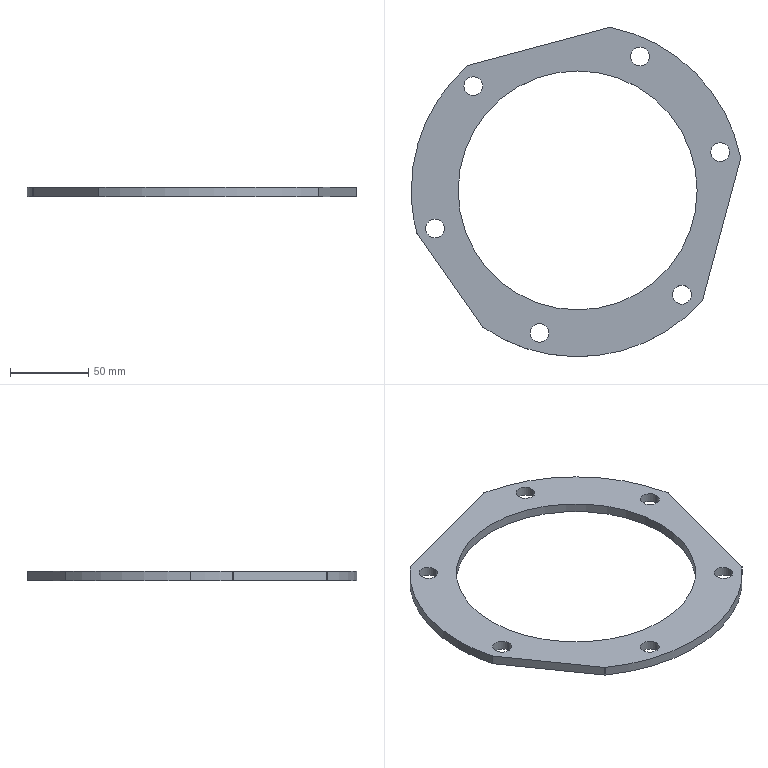Part | SolidWorks | features FlatPattern 1, SMBaseFlange 1, SheetMetal 1 | 1 solid | 29 faces | box 210.92 x 210.92 x 6 mm | volume 89109 mm3 | cylinder 24 | plane 5 | commonest cylinder face diameters 12 x12 2 x6 213 x4 153 x2
STEP:
#1=CARTESIAN_POINT('',(-76.5,0.,6.));
#2=VERTEX_POINT('',#1);
#3=CARTESIAN_POINT('',(76.5,0.,6.));
#4=VERTEX_POINT('',#3);
#5=CARTESIAN_POINT('',(0.,0.,6.));
#6=DIRECTION('',(0.,0.,1.));
#7=DIRECTION('',(1.,0.,0.));
#8=AXIS2_PLACEMENT_3D('',#5,#6,#7);
#9=CIRCLE('',#8,76.5);
#10=EDGE_CURVE('',#2,#4,#9,.T.);
#11=ORIENTED_EDGE('',*,*,#10,.T.);
#12=CARTESIAN_POINT('',(76.5,0.,0.));
#13=VERTEX_POINT('',#12);
#14=CARTESIAN_POINT('',(76.5,0.,6.));
#15=DIRECTION('',(0.,0.,-1.));
#16=VECTOR('',#15,1000.);
#17=LINE('',#14,#16);
#18=EDGE_CURVE('',#4,#13,#17,.T.);
#19=ORIENTED_EDGE('',*,*,#18,.T.);
#20=CARTESIAN_POINT('',(-76.5,0.,0.));
#21=VERTEX_POINT('',#20);
#22=CARTESIAN_POINT('',(0.,0.,0.));
#23=DIRECTION('',(0.,0.,1.));
#24=DIRECTION('',(1.,0.,0.));
#25=AXIS2_PLACEMENT_3D('',#22,#23,#24);
#26=CIRCLE('',#25,76.5);
#27=EDGE_CURVE('',#21,#13,#26,.T.);
#28=ORIENTED_EDGE('',*,*,#27,.F.);
#29=CARTESIAN_POINT('',(-76.5,0.,6.));
#30=DIRECTION('',(0.,0.,-1.));
#31=VECTOR('',#30,1000.);
#32=LINE('',#29,#31);
#33=EDGE_CURVE('',#2,#21,#32,.T.);
#34=ORIENTED_EDGE('',*,*,#33,.F.);
#35=EDGE_LOOP('',(#11,#19,#28,#34));
#36=FACE_OUTER_BOUND('',#35,.T.);
#37=CARTESIAN_POINT('',(0.,0.,6.));
#38=DIRECTION('',(0.,0.,-1.));
#39=DIRECTION('',(-1.,0.,0.));
#40=AXIS2_PLACEMENT_3D('',#37,#38,#39);
#41=CYLINDRICAL_SURFACE('',#40,76.5);
#42=ADVANCED_FACE('',(#36),#41,.F.);
#43=CARTESIAN_POINT('',(-97.28,-24.458,6.));
#44=VERTEX_POINT('',#43);
#45=CARTESIAN_POINT('',(-85.28,-24.458,6.));
#46=VERTEX_POINT('',#45);
#47=CARTESIAN_POINT('',(-91.28,-24.458,6.));
#48=DIRECTION('',(0.,0.,1.));
#49=DIRECTION('',(1.,0.,0.));
#50=AXIS2_PLACEMENT_3D('',#47,#48,#49);
#51=CIRCLE('',#50,6.);
#52=EDGE_CURVE('',#44,#46,#51,.T.);
#53=ORIENTED_EDGE('',*,*,#52,.T.);
#54=CARTESIAN_POINT('',(-85.28,-24.458,0.));
#55=VERTEX_POINT('',#54);
#56=CARTESIAN_POINT('',(-85.28,-24.458,6.));
#57=DIRECTION('',(0.,0.,-1.));
#58=VECTOR('',#57,1000.);
#59=LINE('',#56,#58);
#60=EDGE_CURVE('',#46,#55,#59,.T.);
#61=ORIENTED_EDGE('',*,*,#60,.T.);
#62=CARTESIAN_POINT('',(-97.28,-24.458,0.));
#63=VERTEX_POINT('',#62);
#64=CARTESIAN_POINT('',(-91.28,-24.458,0.));
#65=DIRECTION('',(0.,0.,1.));
#66=DIRECTION('',(1.,0.,0.));
#67=AXIS2_PLACEMENT_3D('',#64,#65,#66);
#68=CIRCLE('',#67,6.);
#69=EDGE_CURVE('',#63,#55,#68,.T.);
#70=ORIENTED_EDGE('',*,*,#69,.F.);
#71=CARTESIAN_POINT('',(-97.28,-24.458,6.));
#72=DIRECTION('',(0.,0.,-1.));
#73=VECTOR('',#72,1000.);
#74=LINE('',#71,#73);
#75=EDGE_CURVE('',#44,#63,#74,.T.);
#76=ORIENTED_EDGE('',*,*,#75,.F.);
#77=EDGE_LOOP('',(#53,#61,#70,#76));
#78=FACE_OUTER_BOUND('',#77,.T.);
#79=CARTESIAN_POINT('',(-91.28,-24.458,6.));
#80=DIRECTION('',(0.,0.,-1.));
#81=DIRECTION('',(-1.,0.,0.));
#82=AXIS2_PLACEMENT_3D('',#79,#80,#81);
#83=CYLINDRICAL_SURFACE('',#82,6.);
#84=ADVANCED_FACE('',(#78),#83,.F.);
#85=CARTESIAN_POINT('',(-30.458,-91.28,6.));
#86=VERTEX_POINT('',#85);
#87=CARTESIAN_POINT('',(-18.458,-91.28,6.));
#88=VERTEX_POINT('',#87);
#89=CARTESIAN_POINT('',(-24.458,-91.28,6.));
#90=DIRECTION('',(0.,0.,1.));
#91=DIRECTION('',(1.,0.,0.));
#92=AXIS2_PLACEMENT_3D('',#89,#90,#91);
#93=CIRCLE('',#92,6.);
#94=EDGE_CURVE('',#86,#88,#93,.T.);
#95=ORIENTED_EDGE('',*,*,#94,.T.);
#96=CARTESIAN_POINT('',(-18.458,-91.28,0.));
#97=VERTEX_POINT('',#96);
#98=CARTESIAN_POINT('',(-18.458,-91.28,6.));
#99=DIRECTION('',(0.,0.,-1.));
#100=VECTOR('',#99,1000.);
#101=LINE('',#98,#100);
#102=EDGE_CURVE('',#88,#97,#101,.T.);
#103=ORIENTED_EDGE('',*,*,#102,.T.);
#104=CARTESIAN_POINT('',(-30.458,-91.28,0.));
#105=VERTEX_POINT('',#104);
#106=CARTESIAN_POINT('',(-24.458,-91.28,0.));
#107=DIRECTION('',(0.,0.,1.));
#108=DIRECTION('',(1.,0.,0.));
#109=AXIS2_PLACEMENT_3D('',#106,#107,#108);
#110=CIRCLE('',#109,6.);
#111=EDGE_CURVE('',#105,#97,#110,.T.);
#112=ORIENTED_EDGE('',*,*,#111,.F.);
#113=CARTESIAN_POINT('',(-30.458,-91.28,6.));
#114=DIRECTION('',(0.,0.,-1.));
#115=VECTOR('',#114,1000.);
#116=LINE('',#113,#115);
#117=EDGE_CURVE('',#86,#105,#116,.T.);
#118=ORIENTED_EDGE('',*,*,#117,.F.);
#119=EDGE_LOOP('',(#95,#103,#112,#118));
#120=FACE_OUTER_BOUND('',#119,.T.);
#121=CARTESIAN_POINT('',(-24.458,-91.28,6.));
#122=DIRECTION('',(0.,0.,-1.));
#123=DIRECTION('',(-1.,0.,0.));
#124=AXIS2_PLACEMENT_3D('',#121,#122,#123);
#125=CYLINDRICAL_SURFACE('',#124,6.);
#126=ADVANCED_FACE('',(#120),#125,.F.);
#127=CARTESIAN_POINT('',(60.822,-66.822,6.));
#128=VERTEX_POINT('',#127);
#129=CARTESIAN_POINT('',(72.822,-66.822,6.));
#130=VERTEX_POINT('',#129);
#131=CARTESIAN_POINT('',(66.822,-66.822,6.));
#132=DIRECTION('',(0.,0.,1.));
#133=DIRECTION('',(1.,0.,0.));
#134=AXIS2_PLACEMENT_3D('',#131,#132,#133);
#135=CIRCLE('',#134,6.);
#136=EDGE_CURVE('',#128,#130,#135,.T.);
#137=ORIENTED_EDGE('',*,*,#136,.T.);
#138=CARTESIAN_POINT('',(72.822,-66.822,0.));
#139=VERTEX_POINT('',#138);
#140=CARTESIAN_POINT('',(72.822,-66.822,6.));
#141=DIRECTION('',(0.,0.,-1.));
#142=VECTOR('',#141,1000.);
#143=LINE('',#140,#142);
#144=EDGE_CURVE('',#130,#139,#143,.T.);
#145=ORIENTED_EDGE('',*,*,#144,.T.);
#146=CARTESIAN_POINT('',(60.822,-66.822,0.));
#147=VERTEX_POINT('',#146);
#148=CARTESIAN_POINT('',(66.822,-66.822,0.));
#149=DIRECTION('',(0.,0.,1.));
#150=DIRECTION('',(1.,0.,0.));
#151=AXIS2_PLACEMENT_3D('',#148,#149,#150);
#152=CIRCLE('',#151,6.);
#153=EDGE_CURVE('',#147,#139,#152,.T.);
#154=ORIENTED_EDGE('',*,*,#153,.F.);
#155=CARTESIAN_POINT('',(60.822,-66.822,6.));
#156=DIRECTION('',(0.,0.,-1.));
#157=VECTOR('',#156,1000.);
#158=LINE('',#155,#157);
#159=EDGE_CURVE('',#128,#147,#158,.T.);
#160=ORIENTED_EDGE('',*,*,#159,.F.);
#161=EDGE_LOOP('',(#137,#145,#154,#160));
#162=FACE_OUTER_BOUND('',#161,.T.);
#163=CARTESIAN_POINT('',(66.822,-66.822,6.));
#164=DIRECTION('',(0.,0.,-1.));
#165=DIRECTION('',(-1.,0.,0.));
#166=AXIS2_PLACEMENT_3D('',#163,#164,#165);
#167=CYLINDRICAL_SURFACE('',#166,6.);
#168=ADVANCED_FACE('',(#162),#167,.F.);
#169=CARTESIAN_POINT('',(85.28,24.458,6.));
#170=VERTEX_POINT('',#169);
#171=CARTESIAN_POINT('',(97.28,24.458,6.));
#172=VERTEX_POINT('',#171);
#173=CARTESIAN_POINT('',(91.28,24.458,6.));
#174=DIRECTION('',(0.,0.,1.));
#175=DIRECTION('',(1.,0.,0.));
#176=AXIS2_PLACEMENT_3D('',#173,#174,#175);
#177=CIRCLE('',#176,6.);
#178=EDGE_CURVE('',#170,#172,#177,.T.);
#179=ORIENTED_EDGE('',*,*,#178,.T.);
#180=CARTESIAN_POINT('',(97.28,24.458,0.));
#181=VERTEX_POINT('',#180);
#182=CARTESIAN_POINT('',(97.28,24.458,6.));
#183=DIRECTION('',(0.,0.,-1.));
#184=VECTOR('',#183,1000.);
#185=LINE('',#182,#184);
#186=EDGE_CURVE('',#172,#181,#185,.T.);
#187=ORIENTED_EDGE('',*,*,#186,.T.);
#188=CARTESIAN_POINT('',(85.28,24.458,0.));
#189=VERTEX_POINT('',#188);
#190=CARTESIAN_POINT('',(91.28,24.458,0.));
#191=DIRECTION('',(0.,0.,1.));
#192=DIRECTION('',(1.,0.,0.));
#193=AXIS2_PLACEMENT_3D('',#190,#191,#192);
#194=CIRCLE('',#193,6.);
#195=EDGE_CURVE('',#189,#181,#194,.T.);
#196=ORIENTED_EDGE('',*,*,#195,.F.);
#197=CARTESIAN_POINT('',(85.28,24.458,6.));
#198=DIRECTION('',(0.,0.,-1.));
#199=VECTOR('',#198,1000.);
#200=LINE('',#197,#199);
#201=EDGE_CURVE('',#170,#189,#200,.T.);
#202=ORIENTED_EDGE('',*,*,#201,.F.);
#203=EDGE_LOOP('',(#179,#187,#196,#202));
#204=FACE_OUTER_BOUND('',#203,.T.);
#205=CARTESIAN_POINT('',(91.28,24.458,6.));
#206=DIRECTION('',(0.,0.,-1.));
#207=DIRECTION('',(-1.,0.,0.));
#208=AXIS2_PLACEMENT_3D('',#205,#206,#207);
#209=CYLINDRICAL_SURFACE('',#208,6.);
#210=ADVANCED_FACE('',(#204),#209,.F.);
#211=CARTESIAN_POINT('',(33.937,85.646,6.));
#212=VERTEX_POINT('',#211);
#213=CARTESIAN_POINT('',(45.937,85.646,6.));
#214=VERTEX_POINT('',#213);
#215=CARTESIAN_POINT('',(39.937,85.646,6.));
#216=DIRECTION('',(0.,0.,1.));
#217=DIRECTION('',(1.,0.,0.));
#218=AXIS2_PLACEMENT_3D('',#215,#216,#217);
#219=CIRCLE('',#218,6.);
#220=EDGE_CURVE('',#212,#214,#219,.T.);
#221=ORIENTED_EDGE('',*,*,#220,.T.);
#222=CARTESIAN_POINT('',(45.937,85.646,0.));
#223=VERTEX_POINT('',#222);
#224=CARTESIAN_POINT('',(45.937,85.646,6.));
#225=DIRECTION('',(0.,0.,-1.));
#226=VECTOR('',#225,1000.);
#227=LINE('',#224,#226);
#228=EDGE_CURVE('',#214,#223,#227,.T.);
#229=ORIENTED_EDGE('',*,*,#228,.T.);
#230=CARTESIAN_POINT('',(33.937,85.646,0.));
#231=VERTEX_POINT('',#230);
#232=CARTESIAN_POINT('',(39.937,85.646,0.));
#233=DIRECTION('',(0.,0.,1.));
#234=DIRECTION('',(1.,0.,0.));
#235=AXIS2_PLACEMENT_3D('',#232,#233,#234);
#236=CIRCLE('',#235,6.);
#237=EDGE_CURVE('',#231,#223,#236,.T.);
#238=ORIENTED_EDGE('',*,*,#237,.F.);
#239=CARTESIAN_POINT('',(33.937,85.646,6.));
#240=DIRECTION('',(0.,0.,-1.));
#241=VECTOR('',#240,1000.);
#242=LINE('',#239,#241);
#243=EDGE_CURVE('',#212,#231,#242,.T.);
#244=ORIENTED_EDGE('',*,*,#243,.F.);
#245=EDGE_LOOP('',(#221,#229,#238,#244));
#246=FACE_OUTER_BOUND('',#245,.T.);
#247=CARTESIAN_POINT('',(39.937,85.646,6.));
#248=DIRECTION('',(0.,0.,-1.));
#249=DIRECTION('',(-1.,0.,0.));
#250=AXIS2_PLACEMENT_3D('',#247,#248,#249);
#251=CYLINDRICAL_SURFACE('',#250,6.);
#252=ADVANCED_FACE('',(#246),#251,.F.);
#253=CARTESIAN_POINT('',(-72.822,66.822,6.));
#254=VERTEX_POINT('',#253);
#255=CARTESIAN_POINT('',(-60.822,66.822,6.));
#256=VERTEX_POINT('',#255);
#257=CARTESIAN_POINT('',(-66.822,66.822,6.));
#258=DIRECTION('',(0.,0.,1.));
#259=DIRECTION('',(1.,0.,0.));
#260=AXIS2_PLACEMENT_3D('',#257,#258,#259);
#261=CIRCLE('',#260,6.);
#262=EDGE_CURVE('',#254,#256,#261,.T.);
#263=ORIENTED_EDGE('',*,*,#262,.T.);
#264=CARTESIAN_POINT('',(-60.822,66.822,0.));
#265=VERTEX_POINT('',#264);
#266=CARTESIAN_POINT('',(-60.822,66.822,6.));
#267=DIRECTION('',(0.,0.,-1.));
#268=VECTOR('',#267,1000.);
#269=LINE('',#266,#268);
#270=EDGE_CURVE('',#256,#265,#269,.T.);
#271=ORIENTED_EDGE('',*,*,#270,.T.);
#272=CARTESIAN_POINT('',(-72.822,66.822,0.));
#273=VERTEX_POINT('',#272);
#274=CARTESIAN_POINT('',(-66.822,66.822,0.));
#275=DIRECTION('',(0.,0.,1.));
#276=DIRECTION('',(1.,0.,0.));
#277=AXIS2_PLACEMENT_3D('',#274,#275,#276);
#278=CIRCLE('',#277,6.);
#279=EDGE_CURVE('',#273,#265,#278,.T.);
#280=ORIENTED_EDGE('',*,*,#279,.F.);
#281=CARTESIAN_POINT('',(-72.822,66.822,6.));
#282=DIRECTION('',(0.,0.,-1.));
#283=VECTOR('',#282,1000.);
#284=LINE('',#281,#283);
#285=EDGE_CURVE('',#254,#273,#284,.T.);
#286=ORIENTED_EDGE('',*,*,#285,.F.);
#287=EDGE_LOOP('',(#263,#271,#280,#286));
#288=FACE_OUTER_BOUND('',#287,.T.);
#289=CARTESIAN_POINT('',(-66.822,66.822,6.));
#290=DIRECTION('',(0.,0.,-1.));
#291=DIRECTION('',(-1.,0.,0.));
#292=AXIS2_PLACEMENT_3D('',#289,#290,#291);
#293=CYLINDRICAL_SURFACE('',#292,6.);
#294=ADVANCED_FACE('',(#288),#293,.F.);
#295=CARTESIAN_POINT('',(-106.5,0.,6.));
#296=VERTEX_POINT('',#295);
#297=CARTESIAN_POINT('',(-102.975,-27.174,6.));
#298=VERTEX_POINT('',#297);
#299=CARTESIAN_POINT('',(0.,0.,6.));
#300=DIRECTION('',(0.,0.,1.));
#301=DIRECTION('',(1.,0.,0.));
#302=AXIS2_PLACEMENT_3D('',#299,#300,#301);
#303=CIRCLE('',#302,106.5);
#304=EDGE_CURVE('',#296,#298,#303,.T.);
#305=ORIENTED_EDGE('',*,*,#304,.F.);
#306=CARTESIAN_POINT('',(-106.5,0.,0.));
#307=VERTEX_POINT('',#306);
#308=CARTESIAN_POINT('',(-106.5,0.,6.));
#309=DIRECTION('',(0.,0.,-1.));
#310=VECTOR('',#309,1000.);
#311=LINE('',#308,#310);
#312=EDGE_CURVE('',#296,#307,#311,.T.);
#313=ORIENTED_EDGE('',*,*,#312,.T.);
#314=CARTESIAN_POINT('',(-102.975,-27.174,0.));
#315=VERTEX_POINT('',#314);
#316=CARTESIAN_POINT('',(0.,0.,0.));
#317=DIRECTION('',(0.,0.,1.));
#318=DIRECTION('',(1.,0.,0.));
#319=AXIS2_PLACEMENT_3D('',#316,#317,#318);
#320=CIRCLE('',#319,106.5);
#321=EDGE_CURVE('',#307,#315,#320,.T.);
#322=ORIENTED_EDGE('',*,*,#321,.T.);
#323=CARTESIAN_POINT('',(-102.975,-27.174,6.));
#324=DIRECTION('',(0.,0.,-1.));
#325=VECTOR('',#324,1000.);
#326=LINE('',#323,#325);
#327=EDGE_CURVE('',#298,#315,#326,.T.);
#328=ORIENTED_EDGE('',*,*,#327,.F.);
#329=EDGE_LOOP('',(#305,#313,#322,#328));
#330=FACE_OUTER_BOUND('',#329,.T.);
#331=CARTESIAN_POINT('',(0.,0.,6.));
#332=DIRECTION('',(0.,0.,-1.));
#333=DIRECTION('',(-1.,0.,0.));
#334=AXIS2_PLACEMENT_3D('',#331,#332,#333);
#335=CYLINDRICAL_SURFACE('',#334,106.5);
#336=ADVANCED_FACE('',(#330),#335,.T.);
#337=ORIENTED_EDGE('',*,*,#52,.F.);
#338=CARTESIAN_POINT('',(-91.28,-24.458,6.));
#339=DIRECTION('',(0.,0.,1.));
#340=DIRECTION('',(1.,0.,0.));
#341=AXIS2_PLACEMENT_3D('',#338,#339,#340);
#342=CIRCLE('',#341,6.);
#343=EDGE_CURVE('',#46,#44,#342,.T.);
#344=ORIENTED_EDGE('',*,*,#343,.F.);
#345=EDGE_LOOP('',(#337,#344));
#346=FACE_BOUND('',#345,.T.);
#347=ORIENTED_EDGE('',*,*,#136,.F.);
#348=CARTESIAN_POINT('',(66.822,-66.822,6.));
#349=DIRECTION('',(0.,0.,1.));
#350=DIRECTION('',(1.,0.,0.));
#351=AXIS2_PLACEMENT_3D('',#348,#349,#350);
#352=CIRCLE('',#351,6.);
#353=EDGE_CURVE('',#130,#128,#352,.T.);
#354=ORIENTED_EDGE('',*,*,#353,.F.);
#355=EDGE_LOOP('',(#347,#354));
#356=FACE_BOUND('',#355,.T.);
#357=ORIENTED_EDGE('',*,*,#220,.F.);
#358=CARTESIAN_POINT('',(39.937,85.646,6.));
#359=DIRECTION('',(0.,0.,1.));
#360=DIRECTION('',(1.,0.,0.));
#361=AXIS2_PLACEMENT_3D('',#358,#359,#360);
#362=CIRCLE('',#361,6.);
#363=EDGE_CURVE('',#214,#212,#362,.T.);
#364=ORIENTED_EDGE('',*,*,#363,.F.);
#365=EDGE_LOOP('',(#357,#364));
#366=FACE_BOUND('',#365,.T.);
#367=CARTESIAN_POINT('',(-70.023,80.106,6.));
#368=VERTEX_POINT('',#367);
#369=CARTESIAN_POINT('',(-70.426,79.89,6.));
#370=VERTEX_POINT('',#369);
#371=CARTESIAN_POINT('',(-69.764,79.14,6.));
#372=DIRECTION('',(0.,0.,1.));
#373=DIRECTION('',(1.,0.,0.));
#374=AXIS2_PLACEMENT_3D('',#371,#372,#373);
#375=CIRCLE('',#374,1.);
#376=EDGE_CURVE('',#368,#370,#375,.T.);
#377=ORIENTED_EDGE('',*,*,#376,.T.);
#378=CARTESIAN_POINT('',(0.,0.,6.));
#379=DIRECTION('',(0.,0.,1.));
#380=DIRECTION('',(1.,0.,0.));
#381=AXIS2_PLACEMENT_3D('',#378,#379,#380);
#382=CIRCLE('',#381,106.5);
#383=EDGE_CURVE('',#370,#296,#382,.T.);
#384=ORIENTED_EDGE('',*,*,#383,.T.);
#385=ORIENTED_EDGE('',*,*,#304,.T.);
#386=CARTESIAN_POINT('',(-102.827,-27.492,6.));
#387=VERTEX_POINT('',#386);
#388=CARTESIAN_POINT('',(-102.008,-26.919,6.));
#389=DIRECTION('',(0.,0.,1.));
#390=DIRECTION('',(1.,0.,0.));
#391=AXIS2_PLACEMENT_3D('',#388,#389,#390);
#392=CIRCLE('',#391,1.);
#393=EDGE_CURVE('',#298,#387,#392,.T.);
#394=ORIENTED_EDGE('',*,*,#393,.T.);
#395=CARTESIAN_POINT('',(-61.003,-87.223,6.));
#396=VERTEX_POINT('',#395);
#397=CARTESIAN_POINT('',(-102.827,-27.492,6.));
#398=DIRECTION('',(0.5736,-0.8192,0.));
#399=VECTOR('',#398,1000.);
#400=LINE('',#397,#399);
#401=EDGE_CURVE('',#387,#396,#400,.T.);
#402=ORIENTED_EDGE('',*,*,#401,.T.);
#403=CARTESIAN_POINT('',(-60.755,-87.471,6.));
#404=VERTEX_POINT('',#403);
#405=CARTESIAN_POINT('',(-60.184,-86.649,6.));
#406=DIRECTION('',(0.,0.,1.));
#407=DIRECTION('',(1.,0.,0.));
#408=AXIS2_PLACEMENT_3D('',#405,#406,#407);
#409=CIRCLE('',#408,1.);
#410=EDGE_CURVE('',#396,#404,#409,.T.);
#411=ORIENTED_EDGE('',*,*,#410,.T.);
#412=CARTESIAN_POINT('',(79.89,-70.426,6.));
#413=VERTEX_POINT('',#412);
#414=CARTESIAN_POINT('',(0.,0.,6.));
#415=DIRECTION('',(0.,0.,1.));
#416=DIRECTION('',(1.,0.,0.));
#417=AXIS2_PLACEMENT_3D('',#414,#415,#416);
#418=CIRCLE('',#417,106.5);
#419=EDGE_CURVE('',#404,#413,#418,.T.);
#420=ORIENTED_EDGE('',*,*,#419,.T.);
#421=CARTESIAN_POINT('',(80.106,-70.023,6.));
#422=VERTEX_POINT('',#421);
#423=CARTESIAN_POINT('',(79.14,-69.764,6.));
#424=DIRECTION('',(0.,0.,1.));
#425=DIRECTION('',(1.,0.,0.));
#426=AXIS2_PLACEMENT_3D('',#423,#424,#425);
#427=CIRCLE('',#426,1.);
#428=EDGE_CURVE('',#413,#422,#427,.T.);
#429=ORIENTED_EDGE('',*,*,#428,.T.);
#430=CARTESIAN_POINT('',(104.386,20.589,6.));
#431=VERTEX_POINT('',#430);
#432=CARTESIAN_POINT('',(80.106,-70.023,6.));
#433=DIRECTION('',(0.2588,0.9659,0.));
#434=VECTOR('',#433,1000.);
#435=LINE('',#432,#434);
#436=EDGE_CURVE('',#422,#431,#435,.T.);
#437=ORIENTED_EDGE('',*,*,#436,.T.);
#438=CARTESIAN_POINT('',(104.4,21.045,6.));
#439=VERTEX_POINT('',#438);
#440=CARTESIAN_POINT('',(103.42,20.848,6.));
#441=DIRECTION('',(0.,0.,1.));
#442=DIRECTION('',(1.,0.,0.));
#443=AXIS2_PLACEMENT_3D('',#440,#441,#442);
#444=CIRCLE('',#443,1.);
#445=EDGE_CURVE('',#431,#439,#444,.T.);
#446=ORIENTED_EDGE('',*,*,#445,.T.);
#447=CARTESIAN_POINT('',(21.045,104.4,6.));
#448=VERTEX_POINT('',#447);
#449=CARTESIAN_POINT('',(0.,0.,6.));
#450=DIRECTION('',(0.,0.,1.));
#451=DIRECTION('',(1.,0.,0.));
#452=AXIS2_PLACEMENT_3D('',#449,#450,#451);
#453=CIRCLE('',#452,106.5);
#454=EDGE_CURVE('',#439,#448,#453,.T.);
#455=ORIENTED_EDGE('',*,*,#454,.T.);
#456=CARTESIAN_POINT('',(20.589,104.386,6.));
#457=VERTEX_POINT('',#456);
#458=CARTESIAN_POINT('',(20.848,103.42,6.));
#459=DIRECTION('',(0.,0.,1.));
#460=DIRECTION('',(1.,0.,0.));
#461=AXIS2_PLACEMENT_3D('',#458,#459,#460);
#462=CIRCLE('',#461,1.);
#463=EDGE_CURVE('',#448,#457,#462,.T.);
#464=ORIENTED_EDGE('',*,*,#463,.T.);
#465=CARTESIAN_POINT('',(20.589,104.386,6.));
#466=DIRECTION('',(-0.9659,-0.2588,0.));
#467=VECTOR('',#466,1000.);
#468=LINE('',#465,#467);
#469=EDGE_CURVE('',#457,#368,#468,.T.);
#470=ORIENTED_EDGE('',*,*,#469,.T.);
#471=EDGE_LOOP('',(#377,#384,#385,#394,#402,#411,#420,#429,#437,#446,#455,#464,#470));
#472=FACE_OUTER_BOUND('',#471,.T.);
#473=ORIENTED_EDGE('',*,*,#262,.F.);
#474=CARTESIAN_POINT('',(-66.822,66.822,6.));
#475=DIRECTION('',(0.,0.,1.));
#476=DIRECTION('',(1.,0.,0.));
#477=AXIS2_PLACEMENT_3D('',#474,#475,#476);
#478=CIRCLE('',#477,6.);
#479=EDGE_CURVE('',#256,#254,#478,.T.);
#480=ORIENTED_EDGE('',*,*,#479,.F.);
#481=EDGE_LOOP('',(#473,#480));
#482=FACE_BOUND('',#481,.T.);
#483=ORIENTED_EDGE('',*,*,#178,.F.);
#484=CARTESIAN_POINT('',(91.28,24.458,6.));
#485=DIRECTION('',(0.,0.,1.));
#486=DIRECTION('',(1.,0.,0.));
#487=AXIS2_PLACEMENT_3D('',#484,#485,#486);
#488=CIRCLE('',#487,6.);
#489=EDGE_CURVE('',#172,#170,#488,.T.);
#490=ORIENTED_EDGE('',*,*,#489,.F.);
#491=EDGE_LOOP('',(#483,#490));
#492=FACE_BOUND('',#491,.T.);
#493=ORIENTED_EDGE('',*,*,#94,.F.);
#494=CARTESIAN_POINT('',(-24.458,-91.28,6.));
#495=DIRECTION('',(0.,0.,1.));
#496=DIRECTION('',(1.,0.,0.));
#497=AXIS2_PLACEMENT_3D('',#494,#495,#496);
#498=CIRCLE('',#497,6.);
#499=EDGE_CURVE('',#88,#86,#498,.T.);
#500=ORIENTED_EDGE('',*,*,#499,.F.);
#501=EDGE_LOOP('',(#493,#500));
#502=FACE_BOUND('',#501,.T.);
#503=ORIENTED_EDGE('',*,*,#10,.F.);
#504=CARTESIAN_POINT('',(0.,0.,6.));
#505=DIRECTION('',(0.,0.,1.));
#506=DIRECTION('',(1.,0.,0.));
#507=AXIS2_PLACEMENT_3D('',#504,#505,#506);
#508=CIRCLE('',#507,76.5);
#509=EDGE_CURVE('',#4,#2,#508,.T.);
#510=ORIENTED_EDGE('',*,*,#509,.F.);
#511=EDGE_LOOP('',(#503,#510));
#512=FACE_BOUND('',#511,.T.);
#513=CARTESIAN_POINT('',(-69.764,79.14,6.));
#514=DIRECTION('',(0.,0.,1.));
#515=DIRECTION('',(1.,0.,0.));
#516=AXIS2_PLACEMENT_3D('',#513,#514,#515);
#517=PLANE('',#516);
#518=ADVANCED_FACE('',(#346,#356,#366,#472,#482,#492,#502,#512),#517,.T.);
#519=CARTESIAN_POINT('',(-70.023,80.106,0.));
#520=VERTEX_POINT('',#519);
#521=CARTESIAN_POINT('',(-70.426,79.89,0.));
#522=VERTEX_POINT('',#521);
#523=CARTESIAN_POINT('',(-69.764,79.14,0.));
#524=DIRECTION('',(0.,0.,1.));
#525=DIRECTION('',(1.,0.,0.));
#526=AXIS2_PLACEMENT_3D('',#523,#524,#525);
#527=CIRCLE('',#526,1.);
#528=EDGE_CURVE('',#520,#522,#527,.T.);
#529=ORIENTED_EDGE('',*,*,#528,.F.);
#530=CARTESIAN_POINT('',(20.589,104.386,0.));
#531=VERTEX_POINT('',#530);
#532=CARTESIAN_POINT('',(20.589,104.386,0.));
#533=DIRECTION('',(-0.9659,-0.2588,0.));
#534=VECTOR('',#533,1000.);
#535=LINE('',#532,#534);
#536=EDGE_CURVE('',#531,#520,#535,.T.);
#537=ORIENTED_EDGE('',*,*,#536,.F.);
#538=CARTESIAN_POINT('',(21.045,104.4,0.));
#539=VERTEX_POINT('',#538);
#540=CARTESIAN_POINT('',(20.848,103.42,0.));
#541=DIRECTION('',(0.,0.,1.));
#542=DIRECTION('',(1.,0.,0.));
#543=AXIS2_PLACEMENT_3D('',#540,#541,#542);
#544=CIRCLE('',#543,1.);
#545=EDGE_CURVE('',#539,#531,#544,.T.);
#546=ORIENTED_EDGE('',*,*,#545,.F.);
#547=CARTESIAN_POINT('',(104.4,21.045,0.));
#548=VERTEX_POINT('',#547);
#549=CARTESIAN_POINT('',(0.,0.,0.));
#550=DIRECTION('',(0.,0.,1.));
#551=DIRECTION('',(1.,0.,0.));
#552=AXIS2_PLACEMENT_3D('',#549,#550,#551);
#553=CIRCLE('',#552,106.5);
#554=EDGE_CURVE('',#548,#539,#553,.T.);
#555=ORIENTED_EDGE('',*,*,#554,.F.);
#556=CARTESIAN_POINT('',(104.386,20.589,0.));
#557=VERTEX_POINT('',#556);
#558=CARTESIAN_POINT('',(103.42,20.848,0.));
#559=DIRECTION('',(0.,0.,1.));
#560=DIRECTION('',(1.,0.,0.));
#561=AXIS2_PLACEMENT_3D('',#558,#559,#560);
#562=CIRCLE('',#561,1.);
#563=EDGE_CURVE('',#557,#548,#562,.T.);
#564=ORIENTED_EDGE('',*,*,#563,.F.);
#565=CARTESIAN_POINT('',(80.106,-70.023,0.));
#566=VERTEX_POINT('',#565);
#567=CARTESIAN_POINT('',(80.106,-70.023,0.));
#568=DIRECTION('',(0.2588,0.9659,0.));
#569=VECTOR('',#568,1000.);
#570=LINE('',#567,#569);
#571=EDGE_CURVE('',#566,#557,#570,.T.);
#572=ORIENTED_EDGE('',*,*,#571,.F.);
#573=CARTESIAN_POINT('',(79.89,-70.426,0.));
#574=VERTEX_POINT('',#573);
#575=CARTESIAN_POINT('',(79.14,-69.764,0.));
#576=DIRECTION('',(0.,0.,1.));
#577=DIRECTION('',(1.,0.,0.));
#578=AXIS2_PLACEMENT_3D('',#575,#576,#577);
#579=CIRCLE('',#578,1.);
#580=EDGE_CURVE('',#574,#566,#579,.T.);
#581=ORIENTED_EDGE('',*,*,#580,.F.);
#582=CARTESIAN_POINT('',(-60.755,-87.471,0.));
#583=VERTEX_POINT('',#582);
#584=CARTESIAN_POINT('',(0.,0.,0.));
#585=DIRECTION('',(0.,0.,1.));
#586=DIRECTION('',(1.,0.,0.));
#587=AXIS2_PLACEMENT_3D('',#584,#585,#586);
#588=CIRCLE('',#587,106.5);
#589=EDGE_CURVE('',#583,#574,#588,.T.);
#590=ORIENTED_EDGE('',*,*,#589,.F.);
#591=CARTESIAN_POINT('',(-61.003,-87.223,0.));
#592=VERTEX_POINT('',#591);
#593=CARTESIAN_POINT('',(-60.184,-86.649,0.));
#594=DIRECTION('',(0.,0.,1.));
#595=DIRECTION('',(1.,0.,0.));
#596=AXIS2_PLACEMENT_3D('',#593,#594,#595);
#597=CIRCLE('',#596,1.);
#598=EDGE_CURVE('',#592,#583,#597,.T.);
#599=ORIENTED_EDGE('',*,*,#598,.F.);
#600=CARTESIAN_POINT('',(-102.827,-27.492,0.));
#601=VERTEX_POINT('',#600);
#602=CARTESIAN_POINT('',(-102.827,-27.492,0.));
#603=DIRECTION('',(0.5736,-0.8192,0.));
#604=VECTOR('',#603,1000.);
#605=LINE('',#602,#604);
#606=EDGE_CURVE('',#601,#592,#605,.T.);
#607=ORIENTED_EDGE('',*,*,#606,.F.);
#608=CARTESIAN_POINT('',(-102.008,-26.919,0.));
#609=DIRECTION('',(0.,0.,1.));
#610=DIRECTION('',(1.,0.,0.));
#611=AXIS2_PLACEMENT_3D('',#608,#609,#610);
#612=CIRCLE('',#611,1.);
#613=EDGE_CURVE('',#315,#601,#612,.T.);
#614=ORIENTED_EDGE('',*,*,#613,.F.);
#615=ORIENTED_EDGE('',*,*,#321,.F.);
#616=CARTESIAN_POINT('',(0.,0.,0.));
#617=DIRECTION('',(0.,0.,1.));
#618=DIRECTION('',(1.,0.,0.));
#619=AXIS2_PLACEMENT_3D('',#616,#617,#618);
#620=CIRCLE('',#619,106.5);
#621=EDGE_CURVE('',#522,#307,#620,.T.);
#622=ORIENTED_EDGE('',*,*,#621,.F.);
#623=EDGE_LOOP('',(#529,#537,#546,#555,#564,#572,#581,#590,#599,#607,#614,#615,#622));
#624=FACE_OUTER_BOUND('',#623,.T.);
#625=ORIENTED_EDGE('',*,*,#279,.T.);
#626=CARTESIAN_POINT('',(-66.822,66.822,0.));
#627=DIRECTION('',(0.,0.,1.));
#628=DIRECTION('',(1.,0.,0.));
#629=AXIS2_PLACEMENT_3D('',#626,#627,#628);
#630=CIRCLE('',#629,6.);
#631=EDGE_CURVE('',#265,#273,#630,.T.);
#632=ORIENTED_EDGE('',*,*,#631,.T.);
#633=EDGE_LOOP('',(#625,#632));
#634=FACE_BOUND('',#633,.T.);
#635=ORIENTED_EDGE('',*,*,#237,.T.);
#636=CARTESIAN_POINT('',(39.937,85.646,0.));
#637=DIRECTION('',(0.,0.,1.));
#638=DIRECTION('',(1.,0.,0.));
#639=AXIS2_PLACEMENT_3D('',#636,#637,#638);
#640=CIRCLE('',#639,6.);
#641=EDGE_CURVE('',#223,#231,#640,.T.);
#642=ORIENTED_EDGE('',*,*,#641,.T.);
#643=EDGE_LOOP('',(#635,#642));
#644=FACE_BOUND('',#643,.T.);
#645=ORIENTED_EDGE('',*,*,#195,.T.);
#646=CARTESIAN_POINT('',(91.28,24.458,0.));
#647=DIRECTION('',(0.,0.,1.));
#648=DIRECTION('',(1.,0.,0.));
#649=AXIS2_PLACEMENT_3D('',#646,#647,#648);
#650=CIRCLE('',#649,6.);
#651=EDGE_CURVE('',#181,#189,#650,.T.);
#652=ORIENTED_EDGE('',*,*,#651,.T.);
#653=EDGE_LOOP('',(#645,#652));
#654=FACE_BOUND('',#653,.T.);
#655=ORIENTED_EDGE('',*,*,#153,.T.);
#656=CARTESIAN_POINT('',(66.822,-66.822,0.));
#657=DIRECTION('',(0.,0.,1.));
#658=DIRECTION('',(1.,0.,0.));
#659=AXIS2_PLACEMENT_3D('',#656,#657,#658);
#660=CIRCLE('',#659,6.);
#661=EDGE_CURVE('',#139,#147,#660,.T.);
#662=ORIENTED_EDGE('',*,*,#661,.T.);
#663=EDGE_LOOP('',(#655,#662));
#664=FACE_BOUND('',#663,.T.);
#665=ORIENTED_EDGE('',*,*,#111,.T.);
#666=CARTESIAN_POINT('',(-24.458,-91.28,0.));
#667=DIRECTION('',(0.,0.,1.));
#668=DIRECTION('',(1.,0.,0.));
#669=AXIS2_PLACEMENT_3D('',#666,#667,#668);
#670=CIRCLE('',#669,6.);
#671=EDGE_CURVE('',#97,#105,#670,.T.);
#672=ORIENTED_EDGE('',*,*,#671,.T.);
#673=EDGE_LOOP('',(#665,#672));
#674=FACE_BOUND('',#673,.T.);
#675=ORIENTED_EDGE('',*,*,#69,.T.);
#676=CARTESIAN_POINT('',(-91.28,-24.458,0.));
#677=DIRECTION('',(0.,0.,1.));
#678=DIRECTION('',(1.,0.,0.));
#679=AXIS2_PLACEMENT_3D('',#676,#677,#678);
#680=CIRCLE('',#679,6.);
#681=EDGE_CURVE('',#55,#63,#680,.T.);
#682=ORIENTED_EDGE('',*,*,#681,.T.);
#683=EDGE_LOOP('',(#675,#682));
#684=FACE_BOUND('',#683,.T.);
#685=ORIENTED_EDGE('',*,*,#27,.T.);
#686=CARTESIAN_POINT('',(0.,0.,0.));
#687=DIRECTION('',(0.,0.,1.));
#688=DIRECTION('',(1.,0.,0.));
#689=AXIS2_PLACEMENT_3D('',#686,#687,#688);
#690=CIRCLE('',#689,76.5);
#691=EDGE_CURVE('',#13,#21,#690,.T.);
#692=ORIENTED_EDGE('',*,*,#691,.T.);
#693=EDGE_LOOP('',(#685,#692));
#694=FACE_BOUND('',#693,.T.);
#695=CARTESIAN_POINT('',(-69.764,79.14,0.));
#696=DIRECTION('',(0.,0.,1.));
#697=DIRECTION('',(1.,0.,0.));
#698=AXIS2_PLACEMENT_3D('',#695,#696,#697);
#699=PLANE('',#698);
#700=ADVANCED_FACE('',(#624,#634,#644,#654,#664,#674,#684,#694),#699,.F.);
#701=ORIENTED_EDGE('',*,*,#528,.T.);
#702=CARTESIAN_POINT('',(-70.426,79.89,6.));
#703=DIRECTION('',(0.,0.,-1.));
#704=VECTOR('',#703,1000.);
#705=LINE('',#702,#704);
#706=EDGE_CURVE('',#370,#522,#705,.T.);
#707=ORIENTED_EDGE('',*,*,#706,.F.);
#708=ORIENTED_EDGE('',*,*,#376,.F.);
#709=CARTESIAN_POINT('',(-70.023,80.106,6.));
#710=DIRECTION('',(0.,0.,-1.));
#711=VECTOR('',#710,1000.);
#712=LINE('',#709,#711);
#713=EDGE_CURVE('',#368,#520,#712,.T.);
#714=ORIENTED_EDGE('',*,*,#713,.T.);
#715=EDGE_LOOP('',(#701,#707,#708,#714));
#716=FACE_OUTER_BOUND('',#715,.T.);
#717=CARTESIAN_POINT('',(-69.764,79.14,6.));
#718=DIRECTION('',(0.,0.,-1.));
#719=DIRECTION('',(-1.,0.,0.));
#720=AXIS2_PLACEMENT_3D('',#717,#718,#719);
#721=CYLINDRICAL_SURFACE('',#720,1.);
#722=ADVANCED_FACE('',(#716),#721,.T.);
#723=ORIENTED_EDGE('',*,*,#312,.F.);
#724=ORIENTED_EDGE('',*,*,#383,.F.);
#725=ORIENTED_EDGE('',*,*,#706,.T.);
#726=ORIENTED_EDGE('',*,*,#621,.T.);
#727=EDGE_LOOP('',(#723,#724,#725,#726));
#728=FACE_OUTER_BOUND('',#727,.T.);
#729=CARTESIAN_POINT('',(0.,0.,6.));
#730=DIRECTION('',(0.,0.,-1.));
#731=DIRECTION('',(-1.,0.,0.));
#732=AXIS2_PLACEMENT_3D('',#729,#730,#731);
#733=CYLINDRICAL_SURFACE('',#732,106.5);
#734=ADVANCED_FACE('',(#728),#733,.T.);
#735=ORIENTED_EDGE('',*,*,#613,.T.);
#736=CARTESIAN_POINT('',(-102.827,-27.492,6.));
#737=DIRECTION('',(0.,0.,-1.));
#738=VECTOR('',#737,1000.);
#739=LINE('',#736,#738);
#740=EDGE_CURVE('',#387,#601,#739,.T.);
#741=ORIENTED_EDGE('',*,*,#740,.F.);
#742=ORIENTED_EDGE('',*,*,#393,.F.);
#743=ORIENTED_EDGE('',*,*,#327,.T.);
#744=EDGE_LOOP('',(#735,#741,#742,#743));
#745=FACE_OUTER_BOUND('',#744,.T.);
#746=CARTESIAN_POINT('',(-102.008,-26.919,6.));
#747=DIRECTION('',(0.,0.,-1.));
#748=DIRECTION('',(-1.,0.,0.));
#749=AXIS2_PLACEMENT_3D('',#746,#747,#748);
#750=CYLINDRICAL_SURFACE('',#749,1.);
#751=ADVANCED_FACE('',(#745),#750,.T.);
#752=ORIENTED_EDGE('',*,*,#606,.T.);
#753=CARTESIAN_POINT('',(-61.003,-87.223,6.));
#754=DIRECTION('',(0.,0.,-1.));
#755=VECTOR('',#754,1000.);
#756=LINE('',#753,#755);
#757=EDGE_CURVE('',#396,#592,#756,.T.);
#758=ORIENTED_EDGE('',*,*,#757,.F.);
#759=ORIENTED_EDGE('',*,*,#401,.F.);
#760=ORIENTED_EDGE('',*,*,#740,.T.);
#761=EDGE_LOOP('',(#752,#758,#759,#760));
#762=FACE_OUTER_BOUND('',#761,.T.);
#763=CARTESIAN_POINT('',(-102.827,-27.492,6.));
#764=DIRECTION('',(0.8192,0.5736,0.));
#765=DIRECTION('',(-0.5736,0.8192,0.));
#766=AXIS2_PLACEMENT_3D('',#763,#764,#765);
#767=PLANE('',#766);
#768=ADVANCED_FACE('',(#762),#767,.F.);
#769=ORIENTED_EDGE('',*,*,#598,.T.);
#770=CARTESIAN_POINT('',(-60.755,-87.471,6.));
#771=DIRECTION('',(0.,0.,-1.));
#772=VECTOR('',#771,1000.);
#773=LINE('',#770,#772);
#774=EDGE_CURVE('',#404,#583,#773,.T.);
#775=ORIENTED_EDGE('',*,*,#774,.F.);
#776=ORIENTED_EDGE('',*,*,#410,.F.);
#777=ORIENTED_EDGE('',*,*,#757,.T.);
#778=EDGE_LOOP('',(#769,#775,#776,#777));
#779=FACE_OUTER_BOUND('',#778,.T.);
#780=CARTESIAN_POINT('',(-60.184,-86.649,6.));
#781=DIRECTION('',(0.,0.,-1.));
#782=DIRECTION('',(-1.,0.,0.));
#783=AXIS2_PLACEMENT_3D('',#780,#781,#782);
#784=CYLINDRICAL_SURFACE('',#783,1.);
#785=ADVANCED_FACE('',(#779),#784,.T.);
#786=ORIENTED_EDGE('',*,*,#589,.T.);
#787=CARTESIAN_POINT('',(79.89,-70.426,6.));
#788=DIRECTION('',(0.,0.,-1.));
#789=VECTOR('',#788,1000.);
#790=LINE('',#787,#789);
#791=EDGE_CURVE('',#413,#574,#790,.T.);
#792=ORIENTED_EDGE('',*,*,#791,.F.);
#793=ORIENTED_EDGE('',*,*,#419,.F.);
#794=ORIENTED_EDGE('',*,*,#774,.T.);
#795=EDGE_LOOP('',(#786,#792,#793,#794));
#796=FACE_OUTER_BOUND('',#795,.T.);
#797=CARTESIAN_POINT('',(0.,0.,6.));
#798=DIRECTION('',(0.,0.,-1.));
#799=DIRECTION('',(-1.,0.,0.));
#800=AXIS2_PLACEMENT_3D('',#797,#798,#799);
#801=CYLINDRICAL_SURFACE('',#800,106.5);
#802=ADVANCED_FACE('',(#796),#801,.T.);
#803=ORIENTED_EDGE('',*,*,#580,.T.);
#804=CARTESIAN_POINT('',(80.106,-70.023,6.));
#805=DIRECTION('',(0.,0.,-1.));
#806=VECTOR('',#805,1000.);
#807=LINE('',#804,#806);
#808=EDGE_CURVE('',#422,#566,#807,.T.);
#809=ORIENTED_EDGE('',*,*,#808,.F.);
#810=ORIENTED_EDGE('',*,*,#428,.F.);
#811=ORIENTED_EDGE('',*,*,#791,.T.);
#812=EDGE_LOOP('',(#803,#809,#810,#811));
#813=FACE_OUTER_BOUND('',#812,.T.);
#814=CARTESIAN_POINT('',(79.14,-69.764,6.));
#815=DIRECTION('',(0.,0.,-1.));
#816=DIRECTION('',(-1.,0.,0.));
#817=AXIS2_PLACEMENT_3D('',#814,#815,#816);
#818=CYLINDRICAL_SURFACE('',#817,1.);
#819=ADVANCED_FACE('',(#813),#818,.T.);
#820=ORIENTED_EDGE('',*,*,#571,.T.);
#821=CARTESIAN_POINT('',(104.386,20.589,6.));
#822=DIRECTION('',(0.,0.,-1.));
#823=VECTOR('',#822,1000.);
#824=LINE('',#821,#823);
#825=EDGE_CURVE('',#431,#557,#824,.T.);
#826=ORIENTED_EDGE('',*,*,#825,.F.);
#827=ORIENTED_EDGE('',*,*,#436,.F.);
#828=ORIENTED_EDGE('',*,*,#808,.T.);
#829=EDGE_LOOP('',(#820,#826,#827,#828));
#830=FACE_OUTER_BOUND('',#829,.T.);
#831=CARTESIAN_POINT('',(80.106,-70.023,6.));
#832=DIRECTION('',(-0.9659,0.2588,0.));
#833=DIRECTION('',(-0.2588,-0.9659,0.));
#834=AXIS2_PLACEMENT_3D('',#831,#832,#833);
#835=PLANE('',#834);
#836=ADVANCED_FACE('',(#830),#835,.F.);
#837=ORIENTED_EDGE('',*,*,#563,.T.);
#838=CARTESIAN_POINT('',(104.4,21.045,6.));
#839=DIRECTION('',(0.,0.,-1.));
#840=VECTOR('',#839,1000.);
#841=LINE('',#838,#840);
#842=EDGE_CURVE('',#439,#548,#841,.T.);
#843=ORIENTED_EDGE('',*,*,#842,.F.);
#844=ORIENTED_EDGE('',*,*,#445,.F.);
#845=ORIENTED_EDGE('',*,*,#825,.T.);
#846=EDGE_LOOP('',(#837,#843,#844,#845));
#847=FACE_OUTER_BOUND('',#846,.T.);
#848=CARTESIAN_POINT('',(103.42,20.848,6.));
#849=DIRECTION('',(0.,0.,-1.));
#850=DIRECTION('',(-1.,0.,0.));
#851=AXIS2_PLACEMENT_3D('',#848,#849,#850);
#852=CYLINDRICAL_SURFACE('',#851,1.);
#853=ADVANCED_FACE('',(#847),#852,.T.);
#854=ORIENTED_EDGE('',*,*,#554,.T.);
#855=CARTESIAN_POINT('',(21.045,104.4,6.));
#856=DIRECTION('',(0.,0.,-1.));
#857=VECTOR('',#856,1000.);
#858=LINE('',#855,#857);
#859=EDGE_CURVE('',#448,#539,#858,.T.);
#860=ORIENTED_EDGE('',*,*,#859,.F.);
#861=ORIENTED_EDGE('',*,*,#454,.F.);
#862=ORIENTED_EDGE('',*,*,#842,.T.);
#863=EDGE_LOOP('',(#854,#860,#861,#862));
#864=FACE_OUTER_BOUND('',#863,.T.);
#865=CARTESIAN_POINT('',(0.,0.,6.));
#866=DIRECTION('',(0.,0.,-1.));
#867=DIRECTION('',(-1.,0.,0.));
#868=AXIS2_PLACEMENT_3D('',#865,#866,#867);
#869=CYLINDRICAL_SURFACE('',#868,106.5);
#870=ADVANCED_FACE('',(#864),#869,.T.);
#871=ORIENTED_EDGE('',*,*,#545,.T.);
#872=CARTESIAN_POINT('',(20.589,104.386,6.));
#873=DIRECTION('',(0.,0.,-1.));
#874=VECTOR('',#873,1000.);
#875=LINE('',#872,#874);
#876=EDGE_CURVE('',#457,#531,#875,.T.);
#877=ORIENTED_EDGE('',*,*,#876,.F.);
#878=ORIENTED_EDGE('',*,*,#463,.F.);
#879=ORIENTED_EDGE('',*,*,#859,.T.);
#880=EDGE_LOOP('',(#871,#877,#878,#879));
#881=FACE_OUTER_BOUND('',#880,.T.);
#882=CARTESIAN_POINT('',(20.848,103.42,6.));
#883=DIRECTION('',(0.,0.,-1.));
#884=DIRECTION('',(-1.,0.,0.));
#885=AXIS2_PLACEMENT_3D('',#882,#883,#884);
#886=CYLINDRICAL_SURFACE('',#885,1.);
#887=ADVANCED_FACE('',(#881),#886,.T.);
#888=ORIENTED_EDGE('',*,*,#536,.T.);
#889=ORIENTED_EDGE('',*,*,#713,.F.);
#890=ORIENTED_EDGE('',*,*,#469,.F.);
#891=ORIENTED_EDGE('',*,*,#876,.T.);
#892=EDGE_LOOP('',(#888,#889,#890,#891));
#893=FACE_OUTER_BOUND('',#892,.T.);
#894=CARTESIAN_POINT('',(20.589,104.386,6.));
#895=DIRECTION('',(0.2588,-0.9659,0.));
#896=DIRECTION('',(0.9659,0.2588,0.));
#897=AXIS2_PLACEMENT_3D('',#894,#895,#896);
#898=PLANE('',#897);
#899=ADVANCED_FACE('',(#893),#898,.F.);
#900=ORIENTED_EDGE('',*,*,#270,.F.);
#901=ORIENTED_EDGE('',*,*,#479,.T.);
#902=ORIENTED_EDGE('',*,*,#285,.T.);
#903=ORIENTED_EDGE('',*,*,#631,.F.);
#904=EDGE_LOOP('',(#900,#901,#902,#903));
#905=FACE_OUTER_BOUND('',#904,.T.);
#906=CARTESIAN_POINT('',(-66.822,66.822,6.));
#907=DIRECTION('',(0.,0.,-1.));
#908=DIRECTION('',(-1.,0.,0.));
#909=AXIS2_PLACEMENT_3D('',#906,#907,#908);
#910=CYLINDRICAL_SURFACE('',#909,6.);
#911=ADVANCED_FACE('',(#905),#910,.F.);
#912=ORIENTED_EDGE('',*,*,#228,.F.);
#913=ORIENTED_EDGE('',*,*,#363,.T.);
#914=ORIENTED_EDGE('',*,*,#243,.T.);
#915=ORIENTED_EDGE('',*,*,#641,.F.);
#916=EDGE_LOOP('',(#912,#913,#914,#915));
#917=FACE_OUTER_BOUND('',#916,.T.);
#918=CARTESIAN_POINT('',(39.937,85.646,6.));
#919=DIRECTION('',(0.,0.,-1.));
#920=DIRECTION('',(-1.,0.,0.));
#921=AXIS2_PLACEMENT_3D('',#918,#919,#920);
#922=CYLINDRICAL_SURFACE('',#921,6.);
#923=ADVANCED_FACE('',(#917),#922,.F.);
#924=ORIENTED_EDGE('',*,*,#186,.F.);
#925=ORIENTED_EDGE('',*,*,#489,.T.);
#926=ORIENTED_EDGE('',*,*,#201,.T.);
#927=ORIENTED_EDGE('',*,*,#651,.F.);
#928=EDGE_LOOP('',(#924,#925,#926,#927));
#929=FACE_OUTER_BOUND('',#928,.T.);
#930=CARTESIAN_POINT('',(91.28,24.458,6.));
#931=DIRECTION('',(0.,0.,-1.));
#932=DIRECTION('',(-1.,0.,0.));
#933=AXIS2_PLACEMENT_3D('',#930,#931,#932);
#934=CYLINDRICAL_SURFACE('',#933,6.);
#935=ADVANCED_FACE('',(#929),#934,.F.);
#936=ORIENTED_EDGE('',*,*,#144,.F.);
#937=ORIENTED_EDGE('',*,*,#353,.T.);
#938=ORIENTED_EDGE('',*,*,#159,.T.);
#939=ORIENTED_EDGE('',*,*,#661,.F.);
#940=EDGE_LOOP('',(#936,#937,#938,#939));
#941=FACE_OUTER_BOUND('',#940,.T.);
#942=CARTESIAN_POINT('',(66.822,-66.822,6.));
#943=DIRECTION('',(0.,0.,-1.));
#944=DIRECTION('',(-1.,0.,0.));
#945=AXIS2_PLACEMENT_3D('',#942,#943,#944);
#946=CYLINDRICAL_SURFACE('',#945,6.);
#947=ADVANCED_FACE('',(#941),#946,.F.);
#948=ORIENTED_EDGE('',*,*,#102,.F.);
#949=ORIENTED_EDGE('',*,*,#499,.T.);
#950=ORIENTED_EDGE('',*,*,#117,.T.);
#951=ORIENTED_EDGE('',*,*,#671,.F.);
#952=EDGE_LOOP('',(#948,#949,#950,#951));
#953=FACE_OUTER_BOUND('',#952,.T.);
#954=CARTESIAN_POINT('',(-24.458,-91.28,6.));
#955=DIRECTION('',(0.,0.,-1.));
#956=DIRECTION('',(-1.,0.,0.));
#957=AXIS2_PLACEMENT_3D('',#954,#955,#956);
#958=CYLINDRICAL_SURFACE('',#957,6.);
#959=ADVANCED_FACE('',(#953),#958,.F.);
#960=ORIENTED_EDGE('',*,*,#60,.F.);
#961=ORIENTED_EDGE('',*,*,#343,.T.);
#962=ORIENTED_EDGE('',*,*,#75,.T.);
#963=ORIENTED_EDGE('',*,*,#681,.F.);
#964=EDGE_LOOP('',(#960,#961,#962,#963));
#965=FACE_OUTER_BOUND('',#964,.T.);
#966=CARTESIAN_POINT('',(-91.28,-24.458,6.));
#967=DIRECTION('',(0.,0.,-1.));
#968=DIRECTION('',(-1.,0.,0.));
#969=AXIS2_PLACEMENT_3D('',#966,#967,#968);
#970=CYLINDRICAL_SURFACE('',#969,6.);
#971=ADVANCED_FACE('',(#965),#970,.F.);
#972=ORIENTED_EDGE('',*,*,#18,.F.);
#973=ORIENTED_EDGE('',*,*,#509,.T.);
#974=ORIENTED_EDGE('',*,*,#33,.T.);
#975=ORIENTED_EDGE('',*,*,#691,.F.);
#976=EDGE_LOOP('',(#972,#973,#974,#975));
#977=FACE_OUTER_BOUND('',#976,.T.);
#978=CARTESIAN_POINT('',(0.,0.,6.));
#979=DIRECTION('',(0.,0.,-1.));
#980=DIRECTION('',(-1.,0.,0.));
#981=AXIS2_PLACEMENT_3D('',#978,#979,#980);
#982=CYLINDRICAL_SURFACE('',#981,76.5);
#983=ADVANCED_FACE('',(#977),#982,.F.);
#984=CLOSED_SHELL('',(#42,#84,#126,#168,#210,#252,#294,#336,#518,#700,#722,#734,#751,#768,#785,#802,#819,#836,#853,#870,#887,#899,#911,#923,#935,#947,#959,#971,#983));
#985=MANIFOLD_SOLID_BREP('',#984);
#986=CARTESIAN_POINT('',(0.,0.,0.));
#987=DIRECTION('',(0.,0.,1.));
#988=DIRECTION('',(1.,0.,0.));
#989=AXIS2_PLACEMENT_3D('',#986,#987,#988);
#990=(LENGTH_UNIT()NAMED_UNIT(*)SI_UNIT(.MILLI.,.METRE.));
#991=UNCERTAINTY_MEASURE_WITH_UNIT(LENGTH_MEASURE(0.00001),#990,'','');
#992=(NAMED_UNIT(*)PLANE_ANGLE_UNIT()SI_UNIT($,.RADIAN.));
#993=(NAMED_UNIT(*)SI_UNIT($,.STERADIAN.)SOLID_ANGLE_UNIT());
#994=(GEOMETRIC_REPRESENTATION_CONTEXT(3)GLOBAL_UNCERTAINTY_ASSIGNED_CONTEXT((#991))GLOBAL_UNIT_ASSIGNED_CONTEXT((#990,#992,#993))REPRESENTATION_CONTEXT('',''));
#995=ADVANCED_BREP_SHAPE_REPRESENTATION('',(#985,#989),#994);